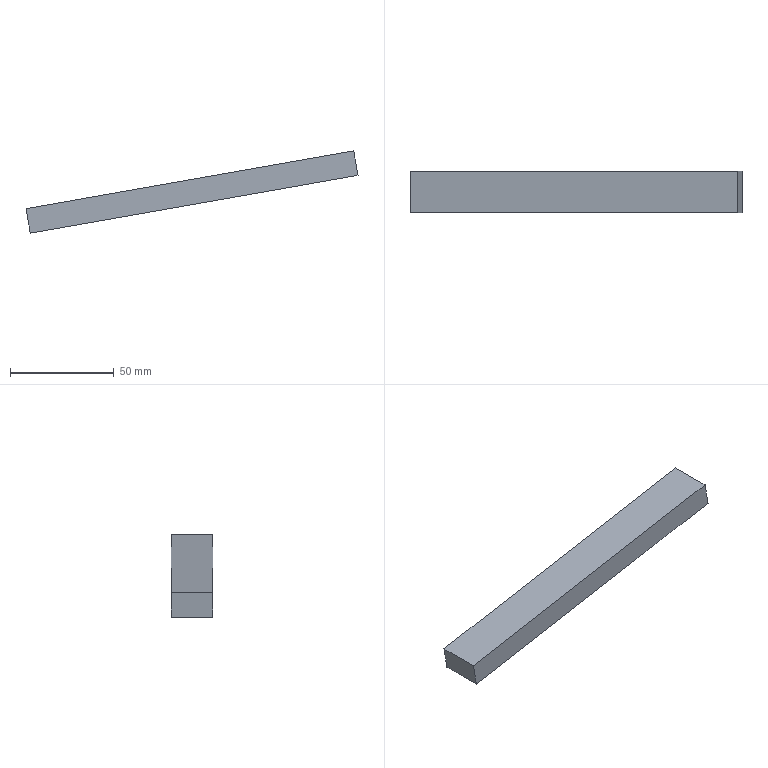Part | NX | features solid 2 | 1 solid | 6 faces | box 159.653 x 20 x 39.601 mm | volume 38400 mm3 | plane 6
STEP:
#1=CARTESIAN_POINT('',(703.754,-485.,132.432));
#2=VERTEX_POINT('',#1);
#3=CARTESIAN_POINT('',(705.838,-485.,120.615));
#4=VERTEX_POINT('',#3);
#5=CARTESIAN_POINT('',(703.754,-485.,132.432));
#6=DIRECTION('',(-0.1736,0.,0.9848));
#7=VECTOR('',#6,1000.);
#8=LINE('',#5,#7);
#9=EDGE_CURVE('',#2,#4,#8,.F.);
#10=ORIENTED_EDGE('',*,*,#9,.F.);
#11=CARTESIAN_POINT('',(861.323,-485.,160.216));
#12=VERTEX_POINT('',#11);
#13=CARTESIAN_POINT('',(871.171,-485.,161.953));
#14=DIRECTION('',(-0.9848,0.,-0.1736));
#15=VECTOR('',#14,1000.);
#16=LINE('',#13,#15);
#17=EDGE_CURVE('',#12,#2,#16,.T.);
#18=ORIENTED_EDGE('',*,*,#17,.F.);
#19=CARTESIAN_POINT('',(863.407,-485.,148.398));
#20=VERTEX_POINT('',#19);
#21=CARTESIAN_POINT('',(861.323,-485.,160.216));
#22=DIRECTION('',(-0.1736,0.,0.9848));
#23=VECTOR('',#22,1000.);
#24=LINE('',#21,#23);
#25=EDGE_CURVE('',#12,#20,#24,.F.);
#26=ORIENTED_EDGE('',*,*,#25,.T.);
#27=CARTESIAN_POINT('',(873.255,-485.,150.135));
#28=DIRECTION('',(0.9848,0.,0.1736));
#29=VECTOR('',#28,1000.);
#30=LINE('',#27,#29);
#31=EDGE_CURVE('',#20,#4,#30,.F.);
#32=ORIENTED_EDGE('',*,*,#31,.T.);
#33=EDGE_LOOP('',(#10,#18,#26,#32));
#34=FACE_BOUND('',#33,.T.);
#35=CARTESIAN_POINT('',(871.171,-485.,161.953));
#36=DIRECTION('',(0.,1.,0.));
#37=DIRECTION('',(-0.9848,0.,-0.1736));
#38=AXIS2_PLACEMENT_3D('',#35,#36,#37);
#39=PLANE('',#38);
#40=ADVANCED_FACE('',(#34),#39,.T.);
#41=CARTESIAN_POINT('',(703.754,-505.,132.432));
#42=VERTEX_POINT('',#41);
#43=CARTESIAN_POINT('',(705.838,-505.,120.615));
#44=VERTEX_POINT('',#43);
#45=CARTESIAN_POINT('',(703.754,-505.,132.432));
#46=DIRECTION('',(0.1736,0.,-0.9848));
#47=VECTOR('',#46,1000.);
#48=LINE('',#45,#47);
#49=EDGE_CURVE('',#42,#44,#48,.T.);
#50=ORIENTED_EDGE('',*,*,#49,.T.);
#51=CARTESIAN_POINT('',(863.407,-505.,148.398));
#52=VERTEX_POINT('',#51);
#53=CARTESIAN_POINT('',(873.255,-505.,150.135));
#54=DIRECTION('',(-0.9848,0.,-0.1736));
#55=VECTOR('',#54,1000.);
#56=LINE('',#53,#55);
#57=EDGE_CURVE('',#52,#44,#56,.T.);
#58=ORIENTED_EDGE('',*,*,#57,.F.);
#59=CARTESIAN_POINT('',(861.323,-505.,160.216));
#60=VERTEX_POINT('',#59);
#61=CARTESIAN_POINT('',(861.323,-505.,160.216));
#62=DIRECTION('',(0.1736,0.,-0.9848));
#63=VECTOR('',#62,1000.);
#64=LINE('',#61,#63);
#65=EDGE_CURVE('',#60,#52,#64,.T.);
#66=ORIENTED_EDGE('',*,*,#65,.F.);
#67=CARTESIAN_POINT('',(871.171,-505.,161.953));
#68=DIRECTION('',(-0.9848,0.,-0.1736));
#69=VECTOR('',#68,1000.);
#70=LINE('',#67,#69);
#71=EDGE_CURVE('',#60,#42,#70,.T.);
#72=ORIENTED_EDGE('',*,*,#71,.T.);
#73=EDGE_LOOP('',(#50,#58,#66,#72));
#74=FACE_BOUND('',#73,.T.);
#75=CARTESIAN_POINT('',(871.171,-505.,161.953));
#76=DIRECTION('',(0.,1.,0.));
#77=DIRECTION('',(-0.9848,0.,-0.1736));
#78=AXIS2_PLACEMENT_3D('',#75,#76,#77);
#79=PLANE('',#78);
#80=ADVANCED_FACE('',(#74),#79,.F.);
#81=ORIENTED_EDGE('',*,*,#31,.F.);
#82=CARTESIAN_POINT('',(863.407,-485.,148.398));
#83=DIRECTION('',(0.,-1.,0.));
#84=VECTOR('',#83,1000.);
#85=LINE('',#82,#84);
#86=EDGE_CURVE('',#20,#52,#85,.T.);
#87=ORIENTED_EDGE('',*,*,#86,.T.);
#88=ORIENTED_EDGE('',*,*,#57,.T.);
#89=CARTESIAN_POINT('',(705.838,-485.,120.615));
#90=DIRECTION('',(0.,-1.,0.));
#91=VECTOR('',#90,1000.);
#92=LINE('',#89,#91);
#93=EDGE_CURVE('',#4,#44,#92,.T.);
#94=ORIENTED_EDGE('',*,*,#93,.F.);
#95=EDGE_LOOP('',(#81,#87,#88,#94));
#96=FACE_BOUND('',#95,.T.);
#97=CARTESIAN_POINT('',(873.255,-485.,150.135));
#98=DIRECTION('',(0.1736,0.,-0.9848));
#99=DIRECTION('',(0.9848,0.,0.1736));
#100=AXIS2_PLACEMENT_3D('',#97,#98,#99);
#101=PLANE('',#100);
#102=ADVANCED_FACE('',(#96),#101,.T.);
#103=CARTESIAN_POINT('',(703.754,-485.,132.432));
#104=DIRECTION('',(0.,-1.,0.));
#105=VECTOR('',#104,1000.);
#106=LINE('',#103,#105);
#107=EDGE_CURVE('',#2,#42,#106,.T.);
#108=ORIENTED_EDGE('',*,*,#107,.T.);
#109=ORIENTED_EDGE('',*,*,#71,.F.);
#110=CARTESIAN_POINT('',(861.323,-485.,160.216));
#111=DIRECTION('',(0.,-1.,0.));
#112=VECTOR('',#111,1000.);
#113=LINE('',#110,#112);
#114=EDGE_CURVE('',#12,#60,#113,.T.);
#115=ORIENTED_EDGE('',*,*,#114,.F.);
#116=ORIENTED_EDGE('',*,*,#17,.T.);
#117=EDGE_LOOP('',(#108,#109,#115,#116));
#118=FACE_BOUND('',#117,.T.);
#119=CARTESIAN_POINT('',(871.171,-485.,161.953));
#120=DIRECTION('',(0.1736,0.,-0.9848));
#121=DIRECTION('',(0.9848,0.,0.1736));
#122=AXIS2_PLACEMENT_3D('',#119,#120,#121);
#123=PLANE('',#122);
#124=ADVANCED_FACE('',(#118),#123,.F.);
#125=ORIENTED_EDGE('',*,*,#25,.F.);
#126=ORIENTED_EDGE('',*,*,#114,.T.);
#127=ORIENTED_EDGE('',*,*,#65,.T.);
#128=ORIENTED_EDGE('',*,*,#86,.F.);
#129=EDGE_LOOP('',(#125,#126,#127,#128));
#130=FACE_BOUND('',#129,.T.);
#131=CARTESIAN_POINT('',(861.323,-485.,160.216));
#132=DIRECTION('',(-0.9848,0.,-0.1736));
#133=DIRECTION('',(0.,-1.,0.));
#134=AXIS2_PLACEMENT_3D('',#131,#132,#133);
#135=PLANE('',#134);
#136=ADVANCED_FACE('',(#130),#135,.F.);
#137=ORIENTED_EDGE('',*,*,#9,.T.);
#138=ORIENTED_EDGE('',*,*,#93,.T.);
#139=ORIENTED_EDGE('',*,*,#49,.F.);
#140=ORIENTED_EDGE('',*,*,#107,.F.);
#141=EDGE_LOOP('',(#137,#138,#139,#140));
#142=FACE_BOUND('',#141,.T.);
#143=CARTESIAN_POINT('',(703.754,-485.,132.432));
#144=DIRECTION('',(-0.9848,0.,-0.1736));
#145=DIRECTION('',(0.,-1.,0.));
#146=AXIS2_PLACEMENT_3D('',#143,#144,#145);
#147=PLANE('',#146);
#148=ADVANCED_FACE('',(#142),#147,.T.);
#149=CLOSED_SHELL('',(#40,#80,#102,#124,#136,#148));
#150=MANIFOLD_SOLID_BREP('',#149);
#151=(LENGTH_UNIT()NAMED_UNIT(*)SI_UNIT(.MILLI.,.METRE.));
#152=UNCERTAINTY_MEASURE_WITH_UNIT(LENGTH_MEASURE(0.00001),#151,'','');
#153=(NAMED_UNIT(*)PLANE_ANGLE_UNIT()SI_UNIT($,.RADIAN.));
#154=(NAMED_UNIT(*)SI_UNIT($,.STERADIAN.)SOLID_ANGLE_UNIT());
#155=(GEOMETRIC_REPRESENTATION_CONTEXT(3)GLOBAL_UNCERTAINTY_ASSIGNED_CONTEXT((#152))GLOBAL_UNIT_ASSIGNED_CONTEXT((#151,#153,#154))REPRESENTATION_CONTEXT('',''));
#156=ADVANCED_BREP_SHAPE_REPRESENTATION('',(#150),#155);